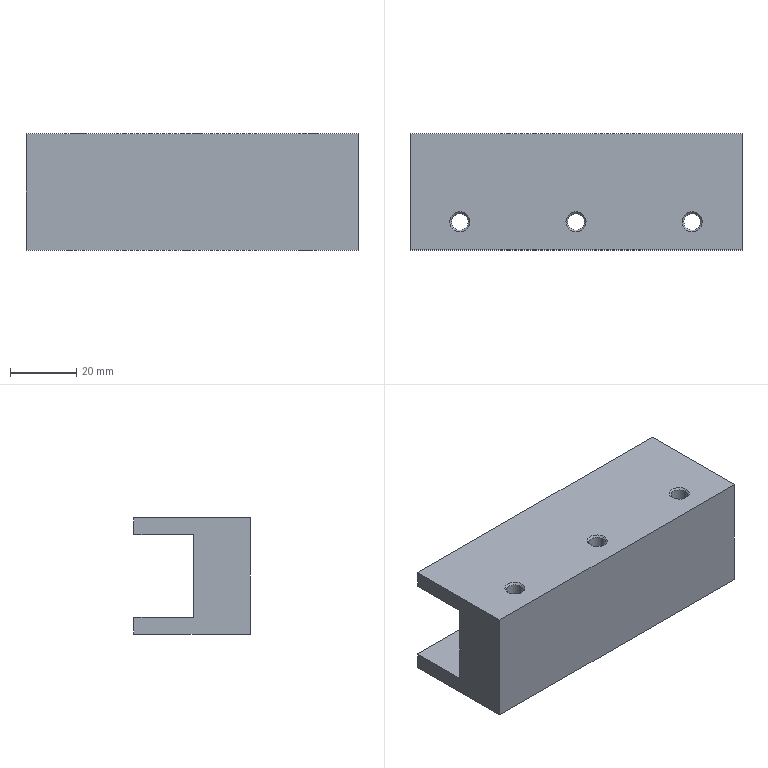Part | SolidWorks | features BaseBody 1 | 1 solid | 22 faces | box 100 x 35 x 35 mm | volume 75431 mm3 | plane 10 | cone 6 | cylinder 6 | commonest cylinder face diameters 5 x6
STEP:
#1=CARTESIAN_POINT('',(-37.5,8.5,-0.525));
#2=VERTEX_POINT('',#1);
#3=CARTESIAN_POINT('',(-32.5,8.5,-0.525));
#4=VERTEX_POINT('',#3);
#5=CARTESIAN_POINT('',(-35.,8.5,-0.525));
#6=DIRECTION('',(0.,0.,1.));
#7=DIRECTION('',(1.,0.,0.));
#8=AXIS2_PLACEMENT_3D('',#5,#6,#7);
#9=CIRCLE('',#8,2.5);
#10=EDGE_CURVE('',#2,#4,#9,.T.);
#11=ORIENTED_EDGE('',*,*,#10,.F.);
#12=CARTESIAN_POINT('',(-38.025,8.5,0.));
#13=VERTEX_POINT('',#12);
#14=CARTESIAN_POINT('',(-38.025,8.5,0.));
#15=DIRECTION('',(-0.7071,0.,0.7071));
#16=VECTOR('',#15,1000.);
#17=LINE('',#14,#16);
#18=EDGE_CURVE('',#2,#13,#17,.T.);
#19=ORIENTED_EDGE('',*,*,#18,.T.);
#20=CARTESIAN_POINT('',(-31.975,8.5,0.));
#21=VERTEX_POINT('',#20);
#22=CARTESIAN_POINT('',(-35.,8.5,0.));
#23=DIRECTION('',(0.,0.,1.));
#24=DIRECTION('',(1.,0.,0.));
#25=AXIS2_PLACEMENT_3D('',#22,#23,#24);
#26=CIRCLE('',#25,3.025);
#27=EDGE_CURVE('',#13,#21,#26,.T.);
#28=ORIENTED_EDGE('',*,*,#27,.T.);
#29=CARTESIAN_POINT('',(-31.975,8.5,0.));
#30=DIRECTION('',(0.7071,0.,0.7071));
#31=VECTOR('',#30,1000.);
#32=LINE('',#29,#31);
#33=EDGE_CURVE('',#4,#21,#32,.T.);
#34=ORIENTED_EDGE('',*,*,#33,.F.);
#35=EDGE_LOOP('',(#11,#19,#28,#34));
#36=FACE_OUTER_BOUND('',#35,.T.);
#37=CARTESIAN_POINT('',(-35.,8.5,0.));
#38=DIRECTION('',(0.,0.,1.));
#39=DIRECTION('',(1.,0.,0.));
#40=AXIS2_PLACEMENT_3D('',#37,#38,#39);
#41=CONICAL_SURFACE('',#40,3.025,0.7854);
#42=ADVANCED_FACE('',(#36),#41,.F.);
#43=CARTESIAN_POINT('',(-37.5,8.5,-35.));
#44=VERTEX_POINT('',#43);
#45=CARTESIAN_POINT('',(-32.5,8.5,-35.));
#46=VERTEX_POINT('',#45);
#47=CARTESIAN_POINT('',(-35.,8.5,-35.));
#48=DIRECTION('',(0.,0.,1.));
#49=DIRECTION('',(1.,0.,0.));
#50=AXIS2_PLACEMENT_3D('',#47,#48,#49);
#51=CIRCLE('',#50,2.5);
#52=EDGE_CURVE('',#44,#46,#51,.T.);
#53=ORIENTED_EDGE('',*,*,#52,.F.);
#54=CARTESIAN_POINT('',(-37.5,8.5,0.));
#55=DIRECTION('',(0.,0.,1.));
#56=VECTOR('',#55,1000.);
#57=LINE('',#54,#56);
#58=EDGE_CURVE('',#44,#2,#57,.T.);
#59=ORIENTED_EDGE('',*,*,#58,.T.);
#60=ORIENTED_EDGE('',*,*,#10,.T.);
#61=CARTESIAN_POINT('',(-32.5,8.5,0.));
#62=DIRECTION('',(0.,0.,1.));
#63=VECTOR('',#62,1000.);
#64=LINE('',#61,#63);
#65=EDGE_CURVE('',#46,#4,#64,.T.);
#66=ORIENTED_EDGE('',*,*,#65,.F.);
#67=EDGE_LOOP('',(#53,#59,#60,#66));
#68=FACE_OUTER_BOUND('',#67,.T.);
#69=CARTESIAN_POINT('',(-35.,8.5,0.));
#70=DIRECTION('',(0.,0.,1.));
#71=DIRECTION('',(1.,0.,0.));
#72=AXIS2_PLACEMENT_3D('',#69,#70,#71);
#73=CYLINDRICAL_SURFACE('',#72,2.5);
#74=ADVANCED_FACE('',(#68),#73,.F.);
#75=CARTESIAN_POINT('',(-2.5,8.5,-0.525));
#76=VERTEX_POINT('',#75);
#77=CARTESIAN_POINT('',(2.5,8.5,-0.525));
#78=VERTEX_POINT('',#77);
#79=CARTESIAN_POINT('',(0.,8.5,-0.525));
#80=DIRECTION('',(0.,0.,1.));
#81=DIRECTION('',(1.,0.,0.));
#82=AXIS2_PLACEMENT_3D('',#79,#80,#81);
#83=CIRCLE('',#82,2.5);
#84=EDGE_CURVE('',#76,#78,#83,.T.);
#85=ORIENTED_EDGE('',*,*,#84,.F.);
#86=CARTESIAN_POINT('',(-3.025,8.5,0.));
#87=VERTEX_POINT('',#86);
#88=CARTESIAN_POINT('',(-3.025,8.5,0.));
#89=DIRECTION('',(-0.7071,0.,0.7071));
#90=VECTOR('',#89,1000.);
#91=LINE('',#88,#90);
#92=EDGE_CURVE('',#76,#87,#91,.T.);
#93=ORIENTED_EDGE('',*,*,#92,.T.);
#94=CARTESIAN_POINT('',(3.025,8.5,0.));
#95=VERTEX_POINT('',#94);
#96=CARTESIAN_POINT('',(0.,8.5,0.));
#97=DIRECTION('',(0.,0.,1.));
#98=DIRECTION('',(1.,0.,0.));
#99=AXIS2_PLACEMENT_3D('',#96,#97,#98);
#100=CIRCLE('',#99,3.025);
#101=EDGE_CURVE('',#87,#95,#100,.T.);
#102=ORIENTED_EDGE('',*,*,#101,.T.);
#103=CARTESIAN_POINT('',(3.025,8.5,0.));
#104=DIRECTION('',(0.7071,0.,0.7071));
#105=VECTOR('',#104,1000.);
#106=LINE('',#103,#105);
#107=EDGE_CURVE('',#78,#95,#106,.T.);
#108=ORIENTED_EDGE('',*,*,#107,.F.);
#109=EDGE_LOOP('',(#85,#93,#102,#108));
#110=FACE_OUTER_BOUND('',#109,.T.);
#111=CARTESIAN_POINT('',(0.,8.5,0.));
#112=DIRECTION('',(0.,0.,1.));
#113=DIRECTION('',(1.,0.,0.));
#114=AXIS2_PLACEMENT_3D('',#111,#112,#113);
#115=CONICAL_SURFACE('',#114,3.025,0.7854);
#116=ADVANCED_FACE('',(#110),#115,.F.);
#117=CARTESIAN_POINT('',(-2.5,8.5,-35.));
#118=VERTEX_POINT('',#117);
#119=CARTESIAN_POINT('',(2.5,8.5,-35.));
#120=VERTEX_POINT('',#119);
#121=CARTESIAN_POINT('',(0.,8.5,-35.));
#122=DIRECTION('',(0.,0.,1.));
#123=DIRECTION('',(1.,0.,0.));
#124=AXIS2_PLACEMENT_3D('',#121,#122,#123);
#125=CIRCLE('',#124,2.5);
#126=EDGE_CURVE('',#118,#120,#125,.T.);
#127=ORIENTED_EDGE('',*,*,#126,.F.);
#128=CARTESIAN_POINT('',(-2.5,8.5,0.));
#129=DIRECTION('',(0.,0.,1.));
#130=VECTOR('',#129,1000.);
#131=LINE('',#128,#130);
#132=EDGE_CURVE('',#118,#76,#131,.T.);
#133=ORIENTED_EDGE('',*,*,#132,.T.);
#134=ORIENTED_EDGE('',*,*,#84,.T.);
#135=CARTESIAN_POINT('',(2.5,8.5,0.));
#136=DIRECTION('',(0.,0.,1.));
#137=VECTOR('',#136,1000.);
#138=LINE('',#135,#137);
#139=EDGE_CURVE('',#120,#78,#138,.T.);
#140=ORIENTED_EDGE('',*,*,#139,.F.);
#141=EDGE_LOOP('',(#127,#133,#134,#140));
#142=FACE_OUTER_BOUND('',#141,.T.);
#143=CARTESIAN_POINT('',(0.,8.5,0.));
#144=DIRECTION('',(0.,0.,1.));
#145=DIRECTION('',(1.,0.,0.));
#146=AXIS2_PLACEMENT_3D('',#143,#144,#145);
#147=CYLINDRICAL_SURFACE('',#146,2.5);
#148=ADVANCED_FACE('',(#142),#147,.F.);
#149=CARTESIAN_POINT('',(32.5,8.5,-0.525));
#150=VERTEX_POINT('',#149);
#151=CARTESIAN_POINT('',(37.5,8.5,-0.525));
#152=VERTEX_POINT('',#151);
#153=CARTESIAN_POINT('',(35.,8.5,-0.525));
#154=DIRECTION('',(0.,0.,1.));
#155=DIRECTION('',(1.,0.,0.));
#156=AXIS2_PLACEMENT_3D('',#153,#154,#155);
#157=CIRCLE('',#156,2.5);
#158=EDGE_CURVE('',#150,#152,#157,.T.);
#159=ORIENTED_EDGE('',*,*,#158,.F.);
#160=CARTESIAN_POINT('',(31.975,8.5,0.));
#161=VERTEX_POINT('',#160);
#162=CARTESIAN_POINT('',(31.975,8.5,0.));
#163=DIRECTION('',(-0.7071,0.,0.7071));
#164=VECTOR('',#163,1000.);
#165=LINE('',#162,#164);
#166=EDGE_CURVE('',#150,#161,#165,.T.);
#167=ORIENTED_EDGE('',*,*,#166,.T.);
#168=CARTESIAN_POINT('',(38.025,8.5,0.));
#169=VERTEX_POINT('',#168);
#170=CARTESIAN_POINT('',(35.,8.5,0.));
#171=DIRECTION('',(0.,0.,1.));
#172=DIRECTION('',(1.,0.,0.));
#173=AXIS2_PLACEMENT_3D('',#170,#171,#172);
#174=CIRCLE('',#173,3.025);
#175=EDGE_CURVE('',#161,#169,#174,.T.);
#176=ORIENTED_EDGE('',*,*,#175,.T.);
#177=CARTESIAN_POINT('',(38.025,8.5,0.));
#178=DIRECTION('',(0.7071,0.,0.7071));
#179=VECTOR('',#178,1000.);
#180=LINE('',#177,#179);
#181=EDGE_CURVE('',#152,#169,#180,.T.);
#182=ORIENTED_EDGE('',*,*,#181,.F.);
#183=EDGE_LOOP('',(#159,#167,#176,#182));
#184=FACE_OUTER_BOUND('',#183,.T.);
#185=CARTESIAN_POINT('',(35.,8.5,0.));
#186=DIRECTION('',(0.,0.,1.));
#187=DIRECTION('',(1.,0.,0.));
#188=AXIS2_PLACEMENT_3D('',#185,#186,#187);
#189=CONICAL_SURFACE('',#188,3.025,0.7854);
#190=ADVANCED_FACE('',(#184),#189,.F.);
#191=CARTESIAN_POINT('',(32.5,8.5,-35.));
#192=VERTEX_POINT('',#191);
#193=CARTESIAN_POINT('',(37.5,8.5,-35.));
#194=VERTEX_POINT('',#193);
#195=CARTESIAN_POINT('',(35.,8.5,-35.));
#196=DIRECTION('',(0.,0.,1.));
#197=DIRECTION('',(1.,0.,0.));
#198=AXIS2_PLACEMENT_3D('',#195,#196,#197);
#199=CIRCLE('',#198,2.5);
#200=EDGE_CURVE('',#192,#194,#199,.T.);
#201=ORIENTED_EDGE('',*,*,#200,.F.);
#202=CARTESIAN_POINT('',(32.5,8.5,0.));
#203=DIRECTION('',(0.,0.,1.));
#204=VECTOR('',#203,1000.);
#205=LINE('',#202,#204);
#206=EDGE_CURVE('',#192,#150,#205,.T.);
#207=ORIENTED_EDGE('',*,*,#206,.T.);
#208=ORIENTED_EDGE('',*,*,#158,.T.);
#209=CARTESIAN_POINT('',(37.5,8.5,0.));
#210=DIRECTION('',(0.,0.,1.));
#211=VECTOR('',#210,1000.);
#212=LINE('',#209,#211);
#213=EDGE_CURVE('',#194,#152,#212,.T.);
#214=ORIENTED_EDGE('',*,*,#213,.F.);
#215=EDGE_LOOP('',(#201,#207,#208,#214));
#216=FACE_OUTER_BOUND('',#215,.T.);
#217=CARTESIAN_POINT('',(35.,8.5,0.));
#218=DIRECTION('',(0.,0.,1.));
#219=DIRECTION('',(1.,0.,0.));
#220=AXIS2_PLACEMENT_3D('',#217,#218,#219);
#221=CYLINDRICAL_SURFACE('',#220,2.5);
#222=ADVANCED_FACE('',(#216),#221,.F.);
#223=CARTESIAN_POINT('',(-50.,17.,-5.));
#224=VERTEX_POINT('',#223);
#225=CARTESIAN_POINT('',(-50.,35.,-5.));
#226=VERTEX_POINT('',#225);
#227=CARTESIAN_POINT('',(-50.,17.,-5.));
#228=DIRECTION('',(0.,1.,0.));
#229=VECTOR('',#228,1000.);
#230=LINE('',#227,#229);
#231=EDGE_CURVE('',#224,#226,#230,.T.);
#232=ORIENTED_EDGE('',*,*,#231,.T.);
#233=CARTESIAN_POINT('',(50.,35.,-5.));
#234=VERTEX_POINT('',#233);
#235=CARTESIAN_POINT('',(50.,35.,-5.));
#236=DIRECTION('',(-1.,0.,0.));
#237=VECTOR('',#236,1000.);
#238=LINE('',#235,#237);
#239=EDGE_CURVE('',#234,#226,#238,.T.);
#240=ORIENTED_EDGE('',*,*,#239,.F.);
#241=CARTESIAN_POINT('',(50.,17.,-5.));
#242=VERTEX_POINT('',#241);
#243=CARTESIAN_POINT('',(50.,17.,-5.));
#244=DIRECTION('',(0.,1.,0.));
#245=VECTOR('',#244,1000.);
#246=LINE('',#243,#245);
#247=EDGE_CURVE('',#242,#234,#246,.T.);
#248=ORIENTED_EDGE('',*,*,#247,.F.);
#249=CARTESIAN_POINT('',(50.,17.,-5.));
#250=DIRECTION('',(-1.,0.,0.));
#251=VECTOR('',#250,1000.);
#252=LINE('',#249,#251);
#253=EDGE_CURVE('',#242,#224,#252,.T.);
#254=ORIENTED_EDGE('',*,*,#253,.T.);
#255=EDGE_LOOP('',(#232,#240,#248,#254));
#256=FACE_OUTER_BOUND('',#255,.T.);
#257=CARTESIAN_POINT('',(50.,17.,-5.));
#258=DIRECTION('',(0.,0.,1.));
#259=DIRECTION('',(1.,0.,0.));
#260=AXIS2_PLACEMENT_3D('',#257,#258,#259);
#261=PLANE('',#260);
#262=ADVANCED_FACE('',(#256),#261,.F.);
#263=CARTESIAN_POINT('',(-50.,35.,0.));
#264=VERTEX_POINT('',#263);
#265=CARTESIAN_POINT('',(-50.,35.,-5.));
#266=DIRECTION('',(0.,0.,1.));
#267=VECTOR('',#266,1000.);
#268=LINE('',#265,#267);
#269=EDGE_CURVE('',#226,#264,#268,.T.);
#270=ORIENTED_EDGE('',*,*,#269,.T.);
#271=CARTESIAN_POINT('',(50.,35.,0.));
#272=VERTEX_POINT('',#271);
#273=CARTESIAN_POINT('',(50.,35.,0.));
#274=DIRECTION('',(-1.,0.,0.));
#275=VECTOR('',#274,1000.);
#276=LINE('',#273,#275);
#277=EDGE_CURVE('',#272,#264,#276,.T.);
#278=ORIENTED_EDGE('',*,*,#277,.F.);
#279=CARTESIAN_POINT('',(50.,35.,-5.));
#280=DIRECTION('',(0.,0.,1.));
#281=VECTOR('',#280,1000.);
#282=LINE('',#279,#281);
#283=EDGE_CURVE('',#234,#272,#282,.T.);
#284=ORIENTED_EDGE('',*,*,#283,.F.);
#285=ORIENTED_EDGE('',*,*,#239,.T.);
#286=EDGE_LOOP('',(#270,#278,#284,#285));
#287=FACE_OUTER_BOUND('',#286,.T.);
#288=CARTESIAN_POINT('',(50.,35.,-5.));
#289=DIRECTION('',(0.,-1.,0.));
#290=DIRECTION('',(0.,0.,-1.));
#291=AXIS2_PLACEMENT_3D('',#288,#289,#290);
#292=PLANE('',#291);
#293=ADVANCED_FACE('',(#287),#292,.F.);
#294=CARTESIAN_POINT('',(-35.,8.5,0.));
#295=DIRECTION('',(0.,0.,1.));
#296=DIRECTION('',(1.,0.,0.));
#297=AXIS2_PLACEMENT_3D('',#294,#295,#296);
#298=CIRCLE('',#297,3.025);
#299=EDGE_CURVE('',#21,#13,#298,.T.);
#300=ORIENTED_EDGE('',*,*,#299,.F.);
#301=ORIENTED_EDGE('',*,*,#27,.F.);
#302=EDGE_LOOP('',(#300,#301));
#303=FACE_BOUND('',#302,.T.);
#304=CARTESIAN_POINT('',(0.,8.5,0.));
#305=DIRECTION('',(0.,0.,1.));
#306=DIRECTION('',(1.,0.,0.));
#307=AXIS2_PLACEMENT_3D('',#304,#305,#306);
#308=CIRCLE('',#307,3.025);
#309=EDGE_CURVE('',#95,#87,#308,.T.);
#310=ORIENTED_EDGE('',*,*,#309,.F.);
#311=ORIENTED_EDGE('',*,*,#101,.F.);
#312=EDGE_LOOP('',(#310,#311));
#313=FACE_BOUND('',#312,.T.);
#314=CARTESIAN_POINT('',(35.,8.5,0.));
#315=DIRECTION('',(0.,0.,1.));
#316=DIRECTION('',(1.,0.,0.));
#317=AXIS2_PLACEMENT_3D('',#314,#315,#316);
#318=CIRCLE('',#317,3.025);
#319=EDGE_CURVE('',#169,#161,#318,.T.);
#320=ORIENTED_EDGE('',*,*,#319,.F.);
#321=ORIENTED_EDGE('',*,*,#175,.F.);
#322=EDGE_LOOP('',(#320,#321));
#323=FACE_BOUND('',#322,.T.);
#324=CARTESIAN_POINT('',(-50.,0.,0.));
#325=VERTEX_POINT('',#324);
#326=CARTESIAN_POINT('',(-50.,35.,0.));
#327=DIRECTION('',(0.,-1.,0.));
#328=VECTOR('',#327,1000.);
#329=LINE('',#326,#328);
#330=EDGE_CURVE('',#264,#325,#329,.T.);
#331=ORIENTED_EDGE('',*,*,#330,.T.);
#332=CARTESIAN_POINT('',(50.,0.,0.));
#333=VERTEX_POINT('',#332);
#334=CARTESIAN_POINT('',(50.,0.,0.));
#335=DIRECTION('',(-1.,0.,0.));
#336=VECTOR('',#335,1000.);
#337=LINE('',#334,#336);
#338=EDGE_CURVE('',#333,#325,#337,.T.);
#339=ORIENTED_EDGE('',*,*,#338,.F.);
#340=CARTESIAN_POINT('',(50.,35.,0.));
#341=DIRECTION('',(0.,-1.,0.));
#342=VECTOR('',#341,1000.);
#343=LINE('',#340,#342);
#344=EDGE_CURVE('',#272,#333,#343,.T.);
#345=ORIENTED_EDGE('',*,*,#344,.F.);
#346=ORIENTED_EDGE('',*,*,#277,.T.);
#347=EDGE_LOOP('',(#331,#339,#345,#346));
#348=FACE_OUTER_BOUND('',#347,.T.);
#349=CARTESIAN_POINT('',(50.,35.,0.));
#350=DIRECTION('',(0.,0.,-1.));
#351=DIRECTION('',(0.,1.,0.));
#352=AXIS2_PLACEMENT_3D('',#349,#350,#351);
#353=PLANE('',#352);
#354=ADVANCED_FACE('',(#303,#313,#323,#348),#353,.F.);
#355=CARTESIAN_POINT('',(-50.,0.,-35.));
#356=VERTEX_POINT('',#355);
#357=CARTESIAN_POINT('',(-50.,0.,0.));
#358=DIRECTION('',(0.,0.,-1.));
#359=VECTOR('',#358,1000.);
#360=LINE('',#357,#359);
#361=EDGE_CURVE('',#325,#356,#360,.T.);
#362=ORIENTED_EDGE('',*,*,#361,.T.);
#363=CARTESIAN_POINT('',(50.,0.,-35.));
#364=VERTEX_POINT('',#363);
#365=CARTESIAN_POINT('',(50.,0.,-35.));
#366=DIRECTION('',(-1.,0.,0.));
#367=VECTOR('',#366,1000.);
#368=LINE('',#365,#367);
#369=EDGE_CURVE('',#364,#356,#368,.T.);
#370=ORIENTED_EDGE('',*,*,#369,.F.);
#371=CARTESIAN_POINT('',(50.,0.,0.));
#372=DIRECTION('',(0.,0.,-1.));
#373=VECTOR('',#372,1000.);
#374=LINE('',#371,#373);
#375=EDGE_CURVE('',#333,#364,#374,.T.);
#376=ORIENTED_EDGE('',*,*,#375,.F.);
#377=ORIENTED_EDGE('',*,*,#338,.T.);
#378=EDGE_LOOP('',(#362,#370,#376,#377));
#379=FACE_OUTER_BOUND('',#378,.T.);
#380=CARTESIAN_POINT('',(50.,0.,0.));
#381=DIRECTION('',(0.,1.,0.));
#382=DIRECTION('',(0.,0.,1.));
#383=AXIS2_PLACEMENT_3D('',#380,#381,#382);
#384=PLANE('',#383);
#385=ADVANCED_FACE('',(#379),#384,.F.);
#386=CARTESIAN_POINT('',(-35.,8.5,-35.));
#387=DIRECTION('',(0.,0.,1.));
#388=DIRECTION('',(1.,0.,0.));
#389=AXIS2_PLACEMENT_3D('',#386,#387,#388);
#390=CIRCLE('',#389,2.5);
#391=EDGE_CURVE('',#46,#44,#390,.T.);
#392=ORIENTED_EDGE('',*,*,#391,.T.);
#393=ORIENTED_EDGE('',*,*,#52,.T.);
#394=EDGE_LOOP('',(#392,#393));
#395=FACE_BOUND('',#394,.T.);
#396=CARTESIAN_POINT('',(0.,8.5,-35.));
#397=DIRECTION('',(0.,0.,1.));
#398=DIRECTION('',(1.,0.,0.));
#399=AXIS2_PLACEMENT_3D('',#396,#397,#398);
#400=CIRCLE('',#399,2.5);
#401=EDGE_CURVE('',#120,#118,#400,.T.);
#402=ORIENTED_EDGE('',*,*,#401,.T.);
#403=ORIENTED_EDGE('',*,*,#126,.T.);
#404=EDGE_LOOP('',(#402,#403));
#405=FACE_BOUND('',#404,.T.);
#406=CARTESIAN_POINT('',(35.,8.5,-35.));
#407=DIRECTION('',(0.,0.,1.));
#408=DIRECTION('',(1.,0.,0.));
#409=AXIS2_PLACEMENT_3D('',#406,#407,#408);
#410=CIRCLE('',#409,2.5);
#411=EDGE_CURVE('',#194,#192,#410,.T.);
#412=ORIENTED_EDGE('',*,*,#411,.T.);
#413=ORIENTED_EDGE('',*,*,#200,.T.);
#414=EDGE_LOOP('',(#412,#413));
#415=FACE_BOUND('',#414,.T.);
#416=CARTESIAN_POINT('',(-50.,35.,-35.));
#417=VERTEX_POINT('',#416);
#418=CARTESIAN_POINT('',(-50.,0.,-35.));
#419=DIRECTION('',(0.,1.,0.));
#420=VECTOR('',#419,1000.);
#421=LINE('',#418,#420);
#422=EDGE_CURVE('',#356,#417,#421,.T.);
#423=ORIENTED_EDGE('',*,*,#422,.T.);
#424=CARTESIAN_POINT('',(50.,35.,-35.));
#425=VERTEX_POINT('',#424);
#426=CARTESIAN_POINT('',(50.,35.,-35.));
#427=DIRECTION('',(-1.,0.,0.));
#428=VECTOR('',#427,1000.);
#429=LINE('',#426,#428);
#430=EDGE_CURVE('',#425,#417,#429,.T.);
#431=ORIENTED_EDGE('',*,*,#430,.F.);
#432=CARTESIAN_POINT('',(50.,0.,-35.));
#433=DIRECTION('',(0.,1.,0.));
#434=VECTOR('',#433,1000.);
#435=LINE('',#432,#434);
#436=EDGE_CURVE('',#364,#425,#435,.T.);
#437=ORIENTED_EDGE('',*,*,#436,.F.);
#438=ORIENTED_EDGE('',*,*,#369,.T.);
#439=EDGE_LOOP('',(#423,#431,#437,#438));
#440=FACE_OUTER_BOUND('',#439,.T.);
#441=CARTESIAN_POINT('',(50.,0.,-35.));
#442=DIRECTION('',(0.,0.,1.));
#443=DIRECTION('',(1.,0.,0.));
#444=AXIS2_PLACEMENT_3D('',#441,#442,#443);
#445=PLANE('',#444);
#446=ADVANCED_FACE('',(#395,#405,#415,#440),#445,.F.);
#447=CARTESIAN_POINT('',(-50.,35.,-30.));
#448=VERTEX_POINT('',#447);
#449=CARTESIAN_POINT('',(-50.,35.,-35.));
#450=DIRECTION('',(0.,0.,1.));
#451=VECTOR('',#450,1000.);
#452=LINE('',#449,#451);
#453=EDGE_CURVE('',#417,#448,#452,.T.);
#454=ORIENTED_EDGE('',*,*,#453,.T.);
#455=CARTESIAN_POINT('',(50.,35.,-30.));
#456=VERTEX_POINT('',#455);
#457=CARTESIAN_POINT('',(50.,35.,-30.));
#458=DIRECTION('',(-1.,0.,0.));
#459=VECTOR('',#458,1000.);
#460=LINE('',#457,#459);
#461=EDGE_CURVE('',#456,#448,#460,.T.);
#462=ORIENTED_EDGE('',*,*,#461,.F.);
#463=CARTESIAN_POINT('',(50.,35.,-35.));
#464=DIRECTION('',(0.,0.,1.));
#465=VECTOR('',#464,1000.);
#466=LINE('',#463,#465);
#467=EDGE_CURVE('',#425,#456,#466,.T.);
#468=ORIENTED_EDGE('',*,*,#467,.F.);
#469=ORIENTED_EDGE('',*,*,#430,.T.);
#470=EDGE_LOOP('',(#454,#462,#468,#469));
#471=FACE_OUTER_BOUND('',#470,.T.);
#472=CARTESIAN_POINT('',(50.,35.,-35.));
#473=DIRECTION('',(0.,-1.,0.));
#474=DIRECTION('',(0.,0.,-1.));
#475=AXIS2_PLACEMENT_3D('',#472,#473,#474);
#476=PLANE('',#475);
#477=ADVANCED_FACE('',(#471),#476,.F.);
#478=CARTESIAN_POINT('',(-50.,17.,-30.));
#479=VERTEX_POINT('',#478);
#480=CARTESIAN_POINT('',(-50.,17.,-30.));
#481=DIRECTION('',(0.,-1.,0.));
#482=VECTOR('',#481,1000.);
#483=LINE('',#480,#482);
#484=EDGE_CURVE('',#448,#479,#483,.T.);
#485=ORIENTED_EDGE('',*,*,#484,.T.);
#486=CARTESIAN_POINT('',(50.,17.,-30.));
#487=VERTEX_POINT('',#486);
#488=CARTESIAN_POINT('',(50.,17.,-30.));
#489=DIRECTION('',(-1.,0.,0.));
#490=VECTOR('',#489,1000.);
#491=LINE('',#488,#490);
#492=EDGE_CURVE('',#487,#479,#491,.T.);
#493=ORIENTED_EDGE('',*,*,#492,.F.);
#494=CARTESIAN_POINT('',(50.,17.,-30.));
#495=DIRECTION('',(0.,-1.,0.));
#496=VECTOR('',#495,1000.);
#497=LINE('',#494,#496);
#498=EDGE_CURVE('',#456,#487,#497,.T.);
#499=ORIENTED_EDGE('',*,*,#498,.F.);
#500=ORIENTED_EDGE('',*,*,#461,.T.);
#501=EDGE_LOOP('',(#485,#493,#499,#500));
#502=FACE_OUTER_BOUND('',#501,.T.);
#503=CARTESIAN_POINT('',(50.,17.,-30.));
#504=DIRECTION('',(0.,0.,-1.));
#505=DIRECTION('',(0.,1.,0.));
#506=AXIS2_PLACEMENT_3D('',#503,#504,#505);
#507=PLANE('',#506);
#508=ADVANCED_FACE('',(#502),#507,.F.);
#509=CARTESIAN_POINT('',(-50.,17.,-5.));
#510=DIRECTION('',(0.,0.,1.));
#511=VECTOR('',#510,1000.);
#512=LINE('',#509,#511);
#513=EDGE_CURVE('',#479,#224,#512,.T.);
#514=ORIENTED_EDGE('',*,*,#513,.T.);
#515=ORIENTED_EDGE('',*,*,#253,.F.);
#516=CARTESIAN_POINT('',(50.,17.,-5.));
#517=DIRECTION('',(0.,0.,1.));
#518=VECTOR('',#517,1000.);
#519=LINE('',#516,#518);
#520=EDGE_CURVE('',#487,#242,#519,.T.);
#521=ORIENTED_EDGE('',*,*,#520,.F.);
#522=ORIENTED_EDGE('',*,*,#492,.T.);
#523=EDGE_LOOP('',(#514,#515,#521,#522));
#524=FACE_OUTER_BOUND('',#523,.T.);
#525=CARTESIAN_POINT('',(50.,17.,-5.));
#526=DIRECTION('',(0.,-1.,0.));
#527=DIRECTION('',(0.,0.,-1.));
#528=AXIS2_PLACEMENT_3D('',#525,#526,#527);
#529=PLANE('',#528);
#530=ADVANCED_FACE('',(#524),#529,.F.);
#531=ORIENTED_EDGE('',*,*,#247,.T.);
#532=ORIENTED_EDGE('',*,*,#283,.T.);
#533=ORIENTED_EDGE('',*,*,#344,.T.);
#534=ORIENTED_EDGE('',*,*,#375,.T.);
#535=ORIENTED_EDGE('',*,*,#436,.T.);
#536=ORIENTED_EDGE('',*,*,#467,.T.);
#537=ORIENTED_EDGE('',*,*,#498,.T.);
#538=ORIENTED_EDGE('',*,*,#520,.T.);
#539=EDGE_LOOP('',(#531,#532,#533,#534,#535,#536,#537,#538));
#540=FACE_OUTER_BOUND('',#539,.T.);
#541=CARTESIAN_POINT('',(50.,0.,0.));
#542=DIRECTION('',(1.,0.,0.));
#543=DIRECTION('',(0.,0.,-1.));
#544=AXIS2_PLACEMENT_3D('',#541,#542,#543);
#545=PLANE('',#544);
#546=ADVANCED_FACE('',(#540),#545,.T.);
#547=ORIENTED_EDGE('',*,*,#231,.F.);
#548=ORIENTED_EDGE('',*,*,#513,.F.);
#549=ORIENTED_EDGE('',*,*,#484,.F.);
#550=ORIENTED_EDGE('',*,*,#453,.F.);
#551=ORIENTED_EDGE('',*,*,#422,.F.);
#552=ORIENTED_EDGE('',*,*,#361,.F.);
#553=ORIENTED_EDGE('',*,*,#330,.F.);
#554=ORIENTED_EDGE('',*,*,#269,.F.);
#555=EDGE_LOOP('',(#547,#548,#549,#550,#551,#552,#553,#554));
#556=FACE_OUTER_BOUND('',#555,.T.);
#557=CARTESIAN_POINT('',(-50.,0.,0.));
#558=DIRECTION('',(1.,0.,0.));
#559=DIRECTION('',(0.,0.,-1.));
#560=AXIS2_PLACEMENT_3D('',#557,#558,#559);
#561=PLANE('',#560);
#562=ADVANCED_FACE('',(#556),#561,.F.);
#563=ORIENTED_EDGE('',*,*,#206,.F.);
#564=ORIENTED_EDGE('',*,*,#411,.F.);
#565=ORIENTED_EDGE('',*,*,#213,.T.);
#566=CARTESIAN_POINT('',(35.,8.5,-0.525));
#567=DIRECTION('',(0.,0.,1.));
#568=DIRECTION('',(1.,0.,0.));
#569=AXIS2_PLACEMENT_3D('',#566,#567,#568);
#570=CIRCLE('',#569,2.5);
#571=EDGE_CURVE('',#152,#150,#570,.T.);
#572=ORIENTED_EDGE('',*,*,#571,.T.);
#573=EDGE_LOOP('',(#563,#564,#565,#572));
#574=FACE_OUTER_BOUND('',#573,.T.);
#575=CARTESIAN_POINT('',(35.,8.5,0.));
#576=DIRECTION('',(0.,0.,1.));
#577=DIRECTION('',(1.,0.,0.));
#578=AXIS2_PLACEMENT_3D('',#575,#576,#577);
#579=CYLINDRICAL_SURFACE('',#578,2.5);
#580=ADVANCED_FACE('',(#574),#579,.F.);
#581=ORIENTED_EDGE('',*,*,#166,.F.);
#582=ORIENTED_EDGE('',*,*,#571,.F.);
#583=ORIENTED_EDGE('',*,*,#181,.T.);
#584=ORIENTED_EDGE('',*,*,#319,.T.);
#585=EDGE_LOOP('',(#581,#582,#583,#584));
#586=FACE_OUTER_BOUND('',#585,.T.);
#587=CARTESIAN_POINT('',(35.,8.5,0.));
#588=DIRECTION('',(0.,0.,1.));
#589=DIRECTION('',(1.,0.,0.));
#590=AXIS2_PLACEMENT_3D('',#587,#588,#589);
#591=CONICAL_SURFACE('',#590,3.025,0.7854);
#592=ADVANCED_FACE('',(#586),#591,.F.);
#593=ORIENTED_EDGE('',*,*,#132,.F.);
#594=ORIENTED_EDGE('',*,*,#401,.F.);
#595=ORIENTED_EDGE('',*,*,#139,.T.);
#596=CARTESIAN_POINT('',(0.,8.5,-0.525));
#597=DIRECTION('',(0.,0.,1.));
#598=DIRECTION('',(1.,0.,0.));
#599=AXIS2_PLACEMENT_3D('',#596,#597,#598);
#600=CIRCLE('',#599,2.5);
#601=EDGE_CURVE('',#78,#76,#600,.T.);
#602=ORIENTED_EDGE('',*,*,#601,.T.);
#603=EDGE_LOOP('',(#593,#594,#595,#602));
#604=FACE_OUTER_BOUND('',#603,.T.);
#605=CARTESIAN_POINT('',(0.,8.5,0.));
#606=DIRECTION('',(0.,0.,1.));
#607=DIRECTION('',(1.,0.,0.));
#608=AXIS2_PLACEMENT_3D('',#605,#606,#607);
#609=CYLINDRICAL_SURFACE('',#608,2.5);
#610=ADVANCED_FACE('',(#604),#609,.F.);
#611=ORIENTED_EDGE('',*,*,#92,.F.);
#612=ORIENTED_EDGE('',*,*,#601,.F.);
#613=ORIENTED_EDGE('',*,*,#107,.T.);
#614=ORIENTED_EDGE('',*,*,#309,.T.);
#615=EDGE_LOOP('',(#611,#612,#613,#614));
#616=FACE_OUTER_BOUND('',#615,.T.);
#617=CARTESIAN_POINT('',(0.,8.5,0.));
#618=DIRECTION('',(0.,0.,1.));
#619=DIRECTION('',(1.,0.,0.));
#620=AXIS2_PLACEMENT_3D('',#617,#618,#619);
#621=CONICAL_SURFACE('',#620,3.025,0.7854);
#622=ADVANCED_FACE('',(#616),#621,.F.);
#623=ORIENTED_EDGE('',*,*,#58,.F.);
#624=ORIENTED_EDGE('',*,*,#391,.F.);
#625=ORIENTED_EDGE('',*,*,#65,.T.);
#626=CARTESIAN_POINT('',(-35.,8.5,-0.525));
#627=DIRECTION('',(0.,0.,1.));
#628=DIRECTION('',(1.,0.,0.));
#629=AXIS2_PLACEMENT_3D('',#626,#627,#628);
#630=CIRCLE('',#629,2.5);
#631=EDGE_CURVE('',#4,#2,#630,.T.);
#632=ORIENTED_EDGE('',*,*,#631,.T.);
#633=EDGE_LOOP('',(#623,#624,#625,#632));
#634=FACE_OUTER_BOUND('',#633,.T.);
#635=CARTESIAN_POINT('',(-35.,8.5,0.));
#636=DIRECTION('',(0.,0.,1.));
#637=DIRECTION('',(1.,0.,0.));
#638=AXIS2_PLACEMENT_3D('',#635,#636,#637);
#639=CYLINDRICAL_SURFACE('',#638,2.5);
#640=ADVANCED_FACE('',(#634),#639,.F.);
#641=ORIENTED_EDGE('',*,*,#18,.F.);
#642=ORIENTED_EDGE('',*,*,#631,.F.);
#643=ORIENTED_EDGE('',*,*,#33,.T.);
#644=ORIENTED_EDGE('',*,*,#299,.T.);
#645=EDGE_LOOP('',(#641,#642,#643,#644));
#646=FACE_OUTER_BOUND('',#645,.T.);
#647=CARTESIAN_POINT('',(-35.,8.5,0.));
#648=DIRECTION('',(0.,0.,1.));
#649=DIRECTION('',(1.,0.,0.));
#650=AXIS2_PLACEMENT_3D('',#647,#648,#649);
#651=CONICAL_SURFACE('',#650,3.025,0.7854);
#652=ADVANCED_FACE('',(#646),#651,.F.);
#653=CLOSED_SHELL('',(#42,#74,#116,#148,#190,#222,#262,#293,#354,#385,#446,#477,#508,#530,#546,#562,#580,#592,#610,#622,#640,#652));
#654=MANIFOLD_SOLID_BREP('',#653);
#655=CARTESIAN_POINT('',(0.,0.,0.));
#656=DIRECTION('',(0.,0.,1.));
#657=DIRECTION('',(1.,0.,0.));
#658=AXIS2_PLACEMENT_3D('',#655,#656,#657);
#659=(LENGTH_UNIT()NAMED_UNIT(*)SI_UNIT(.MILLI.,.METRE.));
#660=UNCERTAINTY_MEASURE_WITH_UNIT(LENGTH_MEASURE(0.00001),#659,'','');
#661=(NAMED_UNIT(*)PLANE_ANGLE_UNIT()SI_UNIT($,.RADIAN.));
#662=(NAMED_UNIT(*)SI_UNIT($,.STERADIAN.)SOLID_ANGLE_UNIT());
#663=(GEOMETRIC_REPRESENTATION_CONTEXT(3)GLOBAL_UNCERTAINTY_ASSIGNED_CONTEXT((#660))GLOBAL_UNIT_ASSIGNED_CONTEXT((#659,#661,#662))REPRESENTATION_CONTEXT('',''));
#664=ADVANCED_BREP_SHAPE_REPRESENTATION('',(#654,#658),#663);